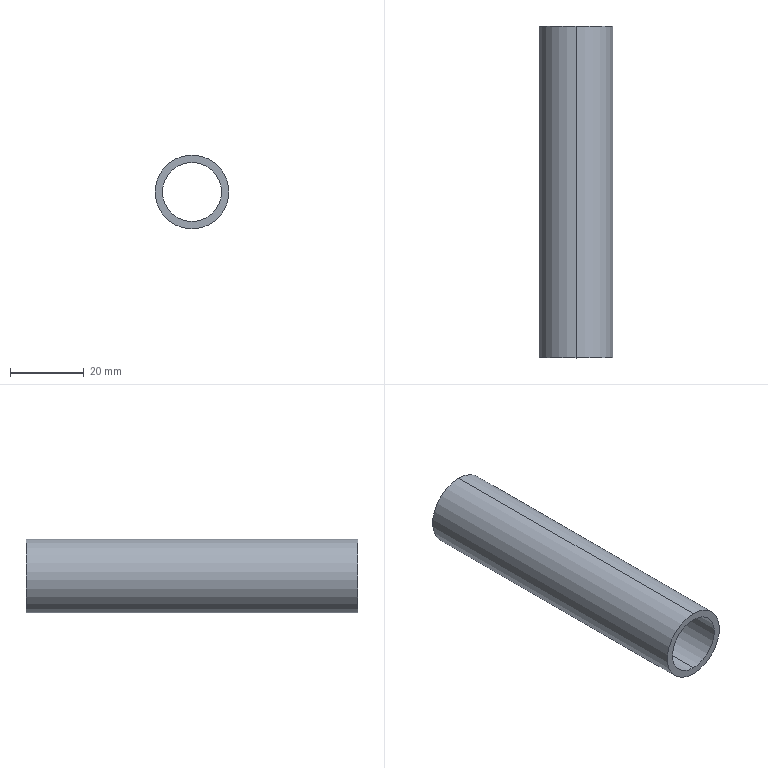Part | SolidWorks | features WeldMemberFeat 1, WeldmentFeature 1 | 1 solid | 6 faces | box 20 x 90 x 20 mm | volume 10179 mm3 | cylinder 4 | plane 2 | commonest cylinder face diameters 16 x2 20 x2
STEP:
#1=CARTESIAN_POINT('',(0.,90.,10.));
#2=VERTEX_POINT('',#1);
#3=CARTESIAN_POINT('',(0.,90.,-10.));
#4=VERTEX_POINT('',#3);
#5=CARTESIAN_POINT('',(0.,90.,0.));
#6=DIRECTION('',(0.,1.,0.));
#7=DIRECTION('',(0.,0.,1.));
#8=AXIS2_PLACEMENT_3D('',#5,#6,#7);
#9=CIRCLE('',#8,10.);
#10=EDGE_CURVE('',#2,#4,#9,.T.);
#11=ORIENTED_EDGE('',*,*,#10,.F.);
#12=CARTESIAN_POINT('',(0.,0.,10.));
#13=VERTEX_POINT('',#12);
#14=CARTESIAN_POINT('',(0.,90.,10.));
#15=DIRECTION('',(0.,-1.,0.));
#16=VECTOR('',#15,1000.);
#17=LINE('',#14,#16);
#18=EDGE_CURVE('',#2,#13,#17,.T.);
#19=ORIENTED_EDGE('',*,*,#18,.T.);
#20=CARTESIAN_POINT('',(0.,0.,-10.));
#21=VERTEX_POINT('',#20);
#22=CARTESIAN_POINT('',(0.,0.,0.));
#23=DIRECTION('',(0.,1.,0.));
#24=DIRECTION('',(0.,0.,1.));
#25=AXIS2_PLACEMENT_3D('',#22,#23,#24);
#26=CIRCLE('',#25,10.);
#27=EDGE_CURVE('',#13,#21,#26,.T.);
#28=ORIENTED_EDGE('',*,*,#27,.T.);
#29=CARTESIAN_POINT('',(0.,90.,-10.));
#30=DIRECTION('',(0.,-1.,0.));
#31=VECTOR('',#30,1000.);
#32=LINE('',#29,#31);
#33=EDGE_CURVE('',#4,#21,#32,.T.);
#34=ORIENTED_EDGE('',*,*,#33,.F.);
#35=EDGE_LOOP('',(#11,#19,#28,#34));
#36=FACE_OUTER_BOUND('',#35,.T.);
#37=CARTESIAN_POINT('',(0.,90.,0.));
#38=DIRECTION('',(0.,-1.,0.));
#39=DIRECTION('',(0.,0.,-1.));
#40=AXIS2_PLACEMENT_3D('',#37,#38,#39);
#41=CYLINDRICAL_SURFACE('',#40,10.);
#42=ADVANCED_FACE('',(#36),#41,.T.);
#43=CARTESIAN_POINT('',(0.,90.,-8.));
#44=VERTEX_POINT('',#43);
#45=CARTESIAN_POINT('',(0.,90.,8.));
#46=VERTEX_POINT('',#45);
#47=CARTESIAN_POINT('',(0.,90.,0.));
#48=DIRECTION('',(0.,1.,0.));
#49=DIRECTION('',(0.,0.,1.));
#50=AXIS2_PLACEMENT_3D('',#47,#48,#49);
#51=CIRCLE('',#50,8.);
#52=EDGE_CURVE('',#44,#46,#51,.T.);
#53=ORIENTED_EDGE('',*,*,#52,.T.);
#54=CARTESIAN_POINT('',(0.,0.,8.));
#55=VERTEX_POINT('',#54);
#56=CARTESIAN_POINT('',(0.,90.,8.));
#57=DIRECTION('',(0.,-1.,0.));
#58=VECTOR('',#57,1000.);
#59=LINE('',#56,#58);
#60=EDGE_CURVE('',#46,#55,#59,.T.);
#61=ORIENTED_EDGE('',*,*,#60,.T.);
#62=CARTESIAN_POINT('',(0.,0.,-8.));
#63=VERTEX_POINT('',#62);
#64=CARTESIAN_POINT('',(0.,0.,0.));
#65=DIRECTION('',(0.,1.,0.));
#66=DIRECTION('',(0.,0.,1.));
#67=AXIS2_PLACEMENT_3D('',#64,#65,#66);
#68=CIRCLE('',#67,8.);
#69=EDGE_CURVE('',#63,#55,#68,.T.);
#70=ORIENTED_EDGE('',*,*,#69,.F.);
#71=CARTESIAN_POINT('',(0.,90.,-8.));
#72=DIRECTION('',(0.,-1.,0.));
#73=VECTOR('',#72,1000.);
#74=LINE('',#71,#73);
#75=EDGE_CURVE('',#44,#63,#74,.T.);
#76=ORIENTED_EDGE('',*,*,#75,.F.);
#77=EDGE_LOOP('',(#53,#61,#70,#76));
#78=FACE_OUTER_BOUND('',#77,.T.);
#79=CARTESIAN_POINT('',(0.,90.,0.));
#80=DIRECTION('',(0.,-1.,0.));
#81=DIRECTION('',(0.,0.,-1.));
#82=AXIS2_PLACEMENT_3D('',#79,#80,#81);
#83=CYLINDRICAL_SURFACE('',#82,8.);
#84=ADVANCED_FACE('',(#78),#83,.F.);
#85=ORIENTED_EDGE('',*,*,#60,.F.);
#86=CARTESIAN_POINT('',(0.,90.,0.));
#87=DIRECTION('',(0.,1.,0.));
#88=DIRECTION('',(0.,0.,1.));
#89=AXIS2_PLACEMENT_3D('',#86,#87,#88);
#90=CIRCLE('',#89,8.);
#91=EDGE_CURVE('',#46,#44,#90,.T.);
#92=ORIENTED_EDGE('',*,*,#91,.T.);
#93=ORIENTED_EDGE('',*,*,#75,.T.);
#94=CARTESIAN_POINT('',(0.,0.,0.));
#95=DIRECTION('',(0.,1.,0.));
#96=DIRECTION('',(0.,0.,1.));
#97=AXIS2_PLACEMENT_3D('',#94,#95,#96);
#98=CIRCLE('',#97,8.);
#99=EDGE_CURVE('',#55,#63,#98,.T.);
#100=ORIENTED_EDGE('',*,*,#99,.F.);
#101=EDGE_LOOP('',(#85,#92,#93,#100));
#102=FACE_OUTER_BOUND('',#101,.T.);
#103=CARTESIAN_POINT('',(0.,90.,0.));
#104=DIRECTION('',(0.,-1.,0.));
#105=DIRECTION('',(0.,0.,-1.));
#106=AXIS2_PLACEMENT_3D('',#103,#104,#105);
#107=CYLINDRICAL_SURFACE('',#106,8.);
#108=ADVANCED_FACE('',(#102),#107,.F.);
#109=ORIENTED_EDGE('',*,*,#18,.F.);
#110=CARTESIAN_POINT('',(0.,90.,0.));
#111=DIRECTION('',(0.,1.,0.));
#112=DIRECTION('',(0.,0.,1.));
#113=AXIS2_PLACEMENT_3D('',#110,#111,#112);
#114=CIRCLE('',#113,10.);
#115=EDGE_CURVE('',#4,#2,#114,.T.);
#116=ORIENTED_EDGE('',*,*,#115,.F.);
#117=ORIENTED_EDGE('',*,*,#33,.T.);
#118=CARTESIAN_POINT('',(0.,0.,0.));
#119=DIRECTION('',(0.,1.,0.));
#120=DIRECTION('',(0.,0.,1.));
#121=AXIS2_PLACEMENT_3D('',#118,#119,#120);
#122=CIRCLE('',#121,10.);
#123=EDGE_CURVE('',#21,#13,#122,.T.);
#124=ORIENTED_EDGE('',*,*,#123,.T.);
#125=EDGE_LOOP('',(#109,#116,#117,#124));
#126=FACE_OUTER_BOUND('',#125,.T.);
#127=CARTESIAN_POINT('',(0.,90.,0.));
#128=DIRECTION('',(0.,-1.,0.));
#129=DIRECTION('',(0.,0.,-1.));
#130=AXIS2_PLACEMENT_3D('',#127,#128,#129);
#131=CYLINDRICAL_SURFACE('',#130,10.);
#132=ADVANCED_FACE('',(#126),#131,.T.);
#133=ORIENTED_EDGE('',*,*,#52,.F.);
#134=ORIENTED_EDGE('',*,*,#91,.F.);
#135=EDGE_LOOP('',(#133,#134));
#136=FACE_BOUND('',#135,.T.);
#137=ORIENTED_EDGE('',*,*,#115,.T.);
#138=ORIENTED_EDGE('',*,*,#10,.T.);
#139=EDGE_LOOP('',(#137,#138));
#140=FACE_OUTER_BOUND('',#139,.T.);
#141=CARTESIAN_POINT('',(0.,90.,0.));
#142=DIRECTION('',(0.,1.,0.));
#143=DIRECTION('',(0.,0.,1.));
#144=AXIS2_PLACEMENT_3D('',#141,#142,#143);
#145=PLANE('',#144);
#146=ADVANCED_FACE('',(#136,#140),#145,.T.);
#147=ORIENTED_EDGE('',*,*,#69,.T.);
#148=ORIENTED_EDGE('',*,*,#99,.T.);
#149=EDGE_LOOP('',(#147,#148));
#150=FACE_BOUND('',#149,.T.);
#151=ORIENTED_EDGE('',*,*,#123,.F.);
#152=ORIENTED_EDGE('',*,*,#27,.F.);
#153=EDGE_LOOP('',(#151,#152));
#154=FACE_OUTER_BOUND('',#153,.T.);
#155=CARTESIAN_POINT('',(0.,0.,0.));
#156=DIRECTION('',(0.,1.,0.));
#157=DIRECTION('',(0.,0.,1.));
#158=AXIS2_PLACEMENT_3D('',#155,#156,#157);
#159=PLANE('',#158);
#160=ADVANCED_FACE('',(#150,#154),#159,.F.);
#161=CLOSED_SHELL('',(#42,#84,#108,#132,#146,#160));
#162=MANIFOLD_SOLID_BREP('',#161);
#163=CARTESIAN_POINT('',(0.,0.,0.));
#164=DIRECTION('',(0.,0.,1.));
#165=DIRECTION('',(1.,0.,0.));
#166=AXIS2_PLACEMENT_3D('',#163,#164,#165);
#167=(LENGTH_UNIT()NAMED_UNIT(*)SI_UNIT(.MILLI.,.METRE.));
#168=UNCERTAINTY_MEASURE_WITH_UNIT(LENGTH_MEASURE(0.00001),#167,'','');
#169=(NAMED_UNIT(*)PLANE_ANGLE_UNIT()SI_UNIT($,.RADIAN.));
#170=(NAMED_UNIT(*)SI_UNIT($,.STERADIAN.)SOLID_ANGLE_UNIT());
#171=(GEOMETRIC_REPRESENTATION_CONTEXT(3)GLOBAL_UNCERTAINTY_ASSIGNED_CONTEXT((#168))GLOBAL_UNIT_ASSIGNED_CONTEXT((#167,#169,#170))REPRESENTATION_CONTEXT('',''));
#172=ADVANCED_BREP_SHAPE_REPRESENTATION('',(#162,#166),#171);